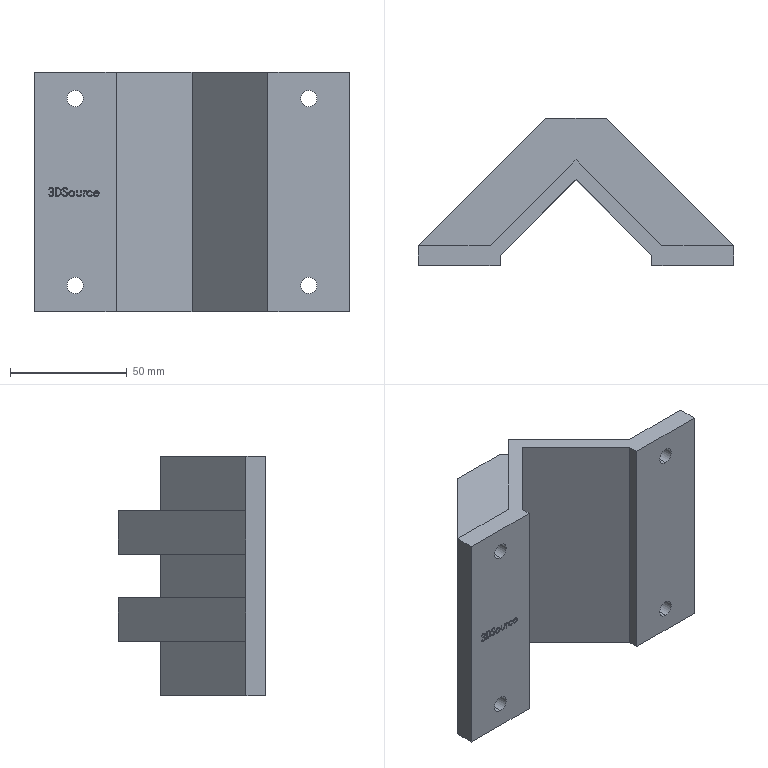Part | NX | features BREP 1 | 1 solid | 115 faces | box 135 x 63 x 102.4 mm | volume 230234 mm3 | plane 76 | cylinder 39 | commonest cylinder face diameters 7 x8 1.458 x7 1.823 x6 2.172 x4 2.552 x4 2.188 x3